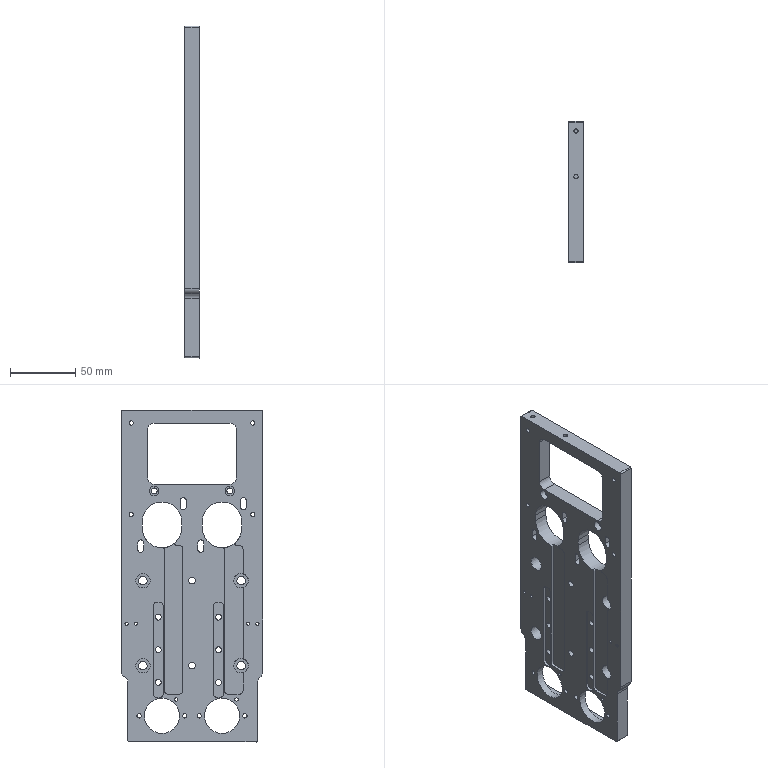Part | 1 solid | 157 faces | box 11 x 108 x 253.9 mm | volume 204420 mm3 | cylinder 96 | plane 61 | commonest cylinder face diameters 4.5 x16 2 x12 3.3 x10 6.07 x8 7.5 x8 10 x8